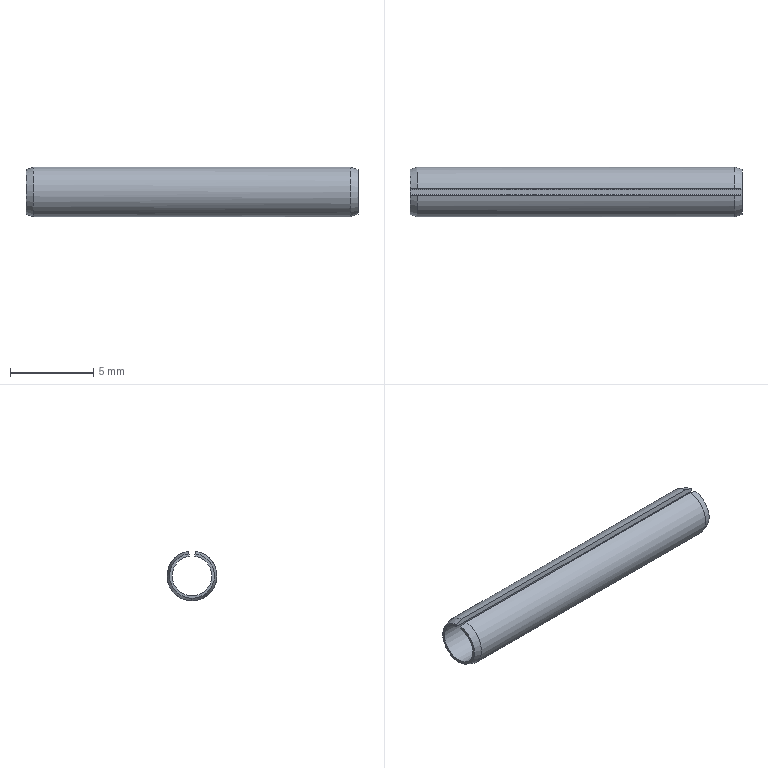Part | STEP file | spring pin slotted light duty1 gb | 1 solid | 9 faces | box 20 x 3 x 2.985 mm | volume 48.044 mm3 | plane 4 | cone 3 | cylinder 2 | commonest cylinder face diameters 2.4 x1 3 x1
STEP:
#1=CARTESIAN_POINT('',(0.,0.,0.));
#2=DIRECTION('',(0.,0.,1.));
#3=DIRECTION('',(1.,0.,0.));
#4=AXIS2_PLACEMENT_3D('',#1,#2,#3);
#5=CARTESIAN_POINT('',(0.,-0.1879,1.337));
#6=VERTEX_POINT('',#5);
#7=CARTESIAN_POINT('',(0.,0.,-1.35));
#8=VERTEX_POINT('',#7);
#9=CARTESIAN_POINT('',(0.,0.,0.));
#10=DIRECTION('',(1.,0.,0.));
#11=DIRECTION('',(0.,0.,-1.));
#12=AXIS2_PLACEMENT_3D('',#9,#10,#11);
#13=CIRCLE('',#12,1.35);
#14=CARTESIAN_POINT('',(0.,0.,0.));
#15=DIRECTION('',(1.,0.,0.));
#16=DIRECTION('',(0.,0.,-1.));
#17=AXIS2_PLACEMENT_3D('',#14,#15,#16);
#18=CONICAL_SURFACE('',#17,1.35,0.3218);
#19=CARTESIAN_POINT('',(0.,0.));
#20=DIRECTION('',(1.,0.));
#21=VECTOR('',#20,1.);
#22=LINE('',#19,#21);
#23=(GEOMETRIC_REPRESENTATION_CONTEXT(2)PARAMETRIC_REPRESENTATION_CONTEXT()REPRESENTATION_CONTEXT('',''));
#24=DEFINITIONAL_REPRESENTATION('',(#22),#23);
#25=PCURVE('',#18,#24);
#26=CARTESIAN_POINT('',(0.,0.,0.));
#27=DIRECTION('',(1.,0.,0.));
#28=DIRECTION('',(0.,0.,-1.));
#29=AXIS2_PLACEMENT_3D('',#26,#27,#28);
#30=PLANE('',#29);
#31=CARTESIAN_POINT('',(0.,0.));
#32=DIRECTION('',(1.,0.));
#33=AXIS2_PLACEMENT_2D('',#31,#32);
#34=CIRCLE('',#33,1.35);
#35=(GEOMETRIC_REPRESENTATION_CONTEXT(2)PARAMETRIC_REPRESENTATION_CONTEXT()REPRESENTATION_CONTEXT('',''));
#36=DEFINITIONAL_REPRESENTATION('',(#34),#35);
#37=PCURVE('',#30,#36);
#38=SURFACE_CURVE('',#13,(#25,#37),.PCURVE_S1.);
#39=EDGE_CURVE('',#6,#8,#38,.T.);
#40=ORIENTED_EDGE('',*,*,#39,.T.);
#41=CARTESIAN_POINT('',(0.45,0.,-1.5));
#42=VERTEX_POINT('',#41);
#43=CARTESIAN_POINT('',(0.,0.,-1.35));
#44=DIRECTION('',(0.9487,0.,-0.3162));
#45=VECTOR('',#44,1.);
#46=LINE('',#43,#45);
#47=CARTESIAN_POINT('',(6.283,0.));
#48=DIRECTION('',(0.,1.));
#49=VECTOR('',#48,1.);
#50=LINE('',#47,#49);
#51=(GEOMETRIC_REPRESENTATION_CONTEXT(2)PARAMETRIC_REPRESENTATION_CONTEXT()REPRESENTATION_CONTEXT('',''));
#52=DEFINITIONAL_REPRESENTATION('',(#50),#51);
#53=PCURVE('',#18,#52);
#54=CARTESIAN_POINT('',(0.,0.,0.));
#55=DIRECTION('',(1.,0.,0.));
#56=DIRECTION('',(0.,0.,-1.));
#57=AXIS2_PLACEMENT_3D('',#54,#55,#56);
#58=CONICAL_SURFACE('',#57,1.35,0.3218);
#59=CARTESIAN_POINT('',(0.,0.));
#60=DIRECTION('',(0.,1.));
#61=VECTOR('',#60,1.);
#62=LINE('',#59,#61);
#63=(GEOMETRIC_REPRESENTATION_CONTEXT(2)PARAMETRIC_REPRESENTATION_CONTEXT()REPRESENTATION_CONTEXT('',''));
#64=DEFINITIONAL_REPRESENTATION('',(#62),#63);
#65=PCURVE('',#58,#64);
#66=SURFACE_CURVE('',#46,(#53,#65),.PCURVE_S1.);
#67=EDGE_CURVE('',#8,#42,#66,.T.);
#68=ORIENTED_EDGE('',*,*,#67,.T.);
#69=CARTESIAN_POINT('',(0.45,-0.2088,1.485));
#70=VERTEX_POINT('',#69);
#71=CARTESIAN_POINT('',(0.45,0.,0.));
#72=DIRECTION('',(1.,0.,0.));
#73=DIRECTION('',(0.,0.,-1.));
#74=AXIS2_PLACEMENT_3D('',#71,#72,#73);
#75=CIRCLE('',#74,1.5);
#76=CARTESIAN_POINT('',(0.,0.45));
#77=DIRECTION('',(1.,0.));
#78=VECTOR('',#77,1.);
#79=LINE('',#76,#78);
#80=(GEOMETRIC_REPRESENTATION_CONTEXT(2)PARAMETRIC_REPRESENTATION_CONTEXT()REPRESENTATION_CONTEXT('',''));
#81=DEFINITIONAL_REPRESENTATION('',(#79),#80);
#82=PCURVE('',#18,#81);
#83=CARTESIAN_POINT('',(20.,0.,0.));
#84=DIRECTION('',(-1.,0.,0.));
#85=DIRECTION('',(0.,0.,1.));
#86=AXIS2_PLACEMENT_3D('',#83,#84,#85);
#87=CYLINDRICAL_SURFACE('',#86,1.5);
#88=CARTESIAN_POINT('',(9.425,19.55));
#89=DIRECTION('',(-1.,0.));
#90=VECTOR('',#89,1.);
#91=LINE('',#88,#90);
#92=(GEOMETRIC_REPRESENTATION_CONTEXT(2)PARAMETRIC_REPRESENTATION_CONTEXT()REPRESENTATION_CONTEXT('',''));
#93=DEFINITIONAL_REPRESENTATION('',(#91),#92);
#94=PCURVE('',#87,#93);
#95=SURFACE_CURVE('',#75,(#82,#94),.PCURVE_S1.);
#96=EDGE_CURVE('',#70,#42,#95,.T.);
#97=ORIENTED_EDGE('',*,*,#96,.F.);
#98=CARTESIAN_POINT('',(-4.05,0.,0.));
#99=DIRECTION('',(0.9487,-0.04401,0.3132));
#100=VECTOR('',#99,1.);
#101=LINE('',#98,#100);
#102=CARTESIAN_POINT('',(3.281,-4.05));
#103=DIRECTION('',(0.,1.));
#104=VECTOR('',#103,1.);
#105=LINE('',#102,#104);
#106=(GEOMETRIC_REPRESENTATION_CONTEXT(2)PARAMETRIC_REPRESENTATION_CONTEXT()REPRESENTATION_CONTEXT('',''));
#107=DEFINITIONAL_REPRESENTATION('',(#105),#106);
#108=PCURVE('',#18,#107);
#109=CARTESIAN_POINT('',(20.,0.,0.));
#110=DIRECTION('',(0.,0.9903,0.1392));
#111=DIRECTION('',(0.,-0.1392,0.9903));
#112=AXIS2_PLACEMENT_3D('',#109,#110,#111);
#113=PLANE('',#112);
#114=CARTESIAN_POINT('',(0.,-24.05));
#115=DIRECTION('',(0.3162,0.9487));
#116=VECTOR('',#115,1.);
#117=LINE('',#114,#116);
#118=(GEOMETRIC_REPRESENTATION_CONTEXT(2)PARAMETRIC_REPRESENTATION_CONTEXT()REPRESENTATION_CONTEXT('',''));
#119=DEFINITIONAL_REPRESENTATION('',(#117),#118);
#120=PCURVE('',#113,#119);
#121=SURFACE_CURVE('',#101,(#108,#120),.PCURVE_S1.);
#122=EDGE_CURVE('',#6,#70,#121,.T.);
#123=ORIENTED_EDGE('',*,*,#122,.F.);
#124=EDGE_LOOP('',(#40,#68,#97,#123));
#125=FACE_BOUND('',#124,.T.);
#126=ADVANCED_FACE('',(#125),#18,.T.);
#127=CARTESIAN_POINT('',(20.,-0.167,1.188));
#128=VERTEX_POINT('',#127);
#129=CARTESIAN_POINT('',(20.,0.167,1.188));
#130=VERTEX_POINT('',#129);
#131=CARTESIAN_POINT('',(20.,0.,0.));
#132=DIRECTION('',(1.,0.,0.));
#133=DIRECTION('',(0.,0.,-1.));
#134=AXIS2_PLACEMENT_3D('',#131,#132,#133);
#135=CIRCLE('',#134,1.2);
#136=CARTESIAN_POINT('',(20.,0.,0.));
#137=DIRECTION('',(1.,0.,0.));
#138=DIRECTION('',(0.,0.,-1.));
#139=AXIS2_PLACEMENT_3D('',#136,#137,#138);
#140=PLANE('',#139);
#141=CARTESIAN_POINT('',(0.,0.));
#142=DIRECTION('',(1.,0.));
#143=AXIS2_PLACEMENT_2D('',#141,#142);
#144=CIRCLE('',#143,1.2);
#145=(GEOMETRIC_REPRESENTATION_CONTEXT(2)PARAMETRIC_REPRESENTATION_CONTEXT()REPRESENTATION_CONTEXT('',''));
#146=DEFINITIONAL_REPRESENTATION('',(#144),#145);
#147=PCURVE('',#140,#146);
#148=CARTESIAN_POINT('',(23.818,0.,0.));
#149=DIRECTION('',(-1.,0.,0.));
#150=DIRECTION('',(0.,0.,1.));
#151=AXIS2_PLACEMENT_3D('',#148,#149,#150);
#152=CYLINDRICAL_SURFACE('',#151,1.2);
#153=CARTESIAN_POINT('',(9.425,3.818));
#154=DIRECTION('',(-1.,0.));
#155=VECTOR('',#154,1.);
#156=LINE('',#153,#155);
#157=(GEOMETRIC_REPRESENTATION_CONTEXT(2)PARAMETRIC_REPRESENTATION_CONTEXT()REPRESENTATION_CONTEXT('',''));
#158=DEFINITIONAL_REPRESENTATION('',(#156),#157);
#159=PCURVE('',#152,#158);
#160=SURFACE_CURVE('',#135,(#147,#159),.PCURVE_S1.);
#161=EDGE_CURVE('',#128,#130,#160,.T.);
#162=ORIENTED_EDGE('',*,*,#161,.F.);
#163=CARTESIAN_POINT('',(20.,-0.1879,1.337));
#164=VERTEX_POINT('',#163);
#165=CARTESIAN_POINT('',(20.,0.,0.));
#166=DIRECTION('',(0.,0.1392,-0.9903));
#167=VECTOR('',#166,1.);
#168=LINE('',#165,#167);
#169=CARTESIAN_POINT('',(0.,0.));
#170=DIRECTION('',(0.9903,0.1392));
#171=VECTOR('',#170,1.);
#172=LINE('',#169,#171);
#173=(GEOMETRIC_REPRESENTATION_CONTEXT(2)PARAMETRIC_REPRESENTATION_CONTEXT()REPRESENTATION_CONTEXT('',''));
#174=DEFINITIONAL_REPRESENTATION('',(#172),#173);
#175=PCURVE('',#140,#174);
#176=CARTESIAN_POINT('',(0.,0.));
#177=DIRECTION('',(-1.,0.));
#178=VECTOR('',#177,1.);
#179=LINE('',#176,#178);
#180=(GEOMETRIC_REPRESENTATION_CONTEXT(2)PARAMETRIC_REPRESENTATION_CONTEXT()REPRESENTATION_CONTEXT('',''));
#181=DEFINITIONAL_REPRESENTATION('',(#179),#180);
#182=PCURVE('',#113,#181);
#183=SURFACE_CURVE('',#168,(#175,#182),.PCURVE_S1.);
#184=EDGE_CURVE('',#164,#128,#183,.T.);
#185=ORIENTED_EDGE('',*,*,#184,.F.);
#186=CARTESIAN_POINT('',(20.,0.1879,1.337));
#187=VERTEX_POINT('',#186);
#188=CARTESIAN_POINT('',(20.,0.,0.));
#189=DIRECTION('',(1.,0.,0.));
#190=DIRECTION('',(0.,0.,-1.));
#191=AXIS2_PLACEMENT_3D('',#188,#189,#190);
#192=CIRCLE('',#191,1.35);
#193=CARTESIAN_POINT('',(0.,0.));
#194=DIRECTION('',(1.,0.));
#195=AXIS2_PLACEMENT_2D('',#193,#194);
#196=CIRCLE('',#195,1.35);
#197=(GEOMETRIC_REPRESENTATION_CONTEXT(2)PARAMETRIC_REPRESENTATION_CONTEXT()REPRESENTATION_CONTEXT('',''));
#198=DEFINITIONAL_REPRESENTATION('',(#196),#197);
#199=PCURVE('',#140,#198);
#200=CARTESIAN_POINT('',(19.55,0.,0.));
#201=DIRECTION('',(-1.,0.,0.));
#202=DIRECTION('',(0.,0.,1.));
#203=AXIS2_PLACEMENT_3D('',#200,#201,#202);
#204=CONICAL_SURFACE('',#203,1.5,0.3218);
#205=CARTESIAN_POINT('',(9.425,-0.45));
#206=DIRECTION('',(-1.,0.));
#207=VECTOR('',#206,1.);
#208=LINE('',#205,#207);
#209=(GEOMETRIC_REPRESENTATION_CONTEXT(2)PARAMETRIC_REPRESENTATION_CONTEXT()REPRESENTATION_CONTEXT('',''));
#210=DEFINITIONAL_REPRESENTATION('',(#208),#209);
#211=PCURVE('',#204,#210);
#212=SURFACE_CURVE('',#192,(#199,#211),.PCURVE_S1.);
#213=EDGE_CURVE('',#164,#187,#212,.T.);
#214=ORIENTED_EDGE('',*,*,#213,.T.);
#215=CARTESIAN_POINT('',(20.,0.,0.));
#216=DIRECTION('',(0.,0.1392,0.9903));
#217=VECTOR('',#216,1.);
#218=LINE('',#215,#217);
#219=CARTESIAN_POINT('',(0.,0.));
#220=DIRECTION('',(-0.9903,0.1392));
#221=VECTOR('',#220,1.);
#222=LINE('',#219,#221);
#223=(GEOMETRIC_REPRESENTATION_CONTEXT(2)PARAMETRIC_REPRESENTATION_CONTEXT()REPRESENTATION_CONTEXT('',''));
#224=DEFINITIONAL_REPRESENTATION('',(#222),#223);
#225=PCURVE('',#140,#224);
#226=CARTESIAN_POINT('',(20.,0.,0.));
#227=DIRECTION('',(0.,-0.9903,0.1392));
#228=DIRECTION('',(0.,-0.1392,-0.9903));
#229=AXIS2_PLACEMENT_3D('',#226,#227,#228);
#230=PLANE('',#229);
#231=CARTESIAN_POINT('',(0.,0.));
#232=DIRECTION('',(-1.,0.));
#233=VECTOR('',#232,1.);
#234=LINE('',#231,#233);
#235=(GEOMETRIC_REPRESENTATION_CONTEXT(2)PARAMETRIC_REPRESENTATION_CONTEXT()REPRESENTATION_CONTEXT('',''));
#236=DEFINITIONAL_REPRESENTATION('',(#234),#235);
#237=PCURVE('',#230,#236);
#238=SURFACE_CURVE('',#218,(#225,#237),.PCURVE_S1.);
#239=EDGE_CURVE('',#130,#187,#238,.T.);
#240=ORIENTED_EDGE('',*,*,#239,.F.);
#241=EDGE_LOOP('',(#162,#185,#214,#240));
#242=FACE_BOUND('',#241,.T.);
#243=ADVANCED_FACE('',(#242),#140,.T.);
#244=CARTESIAN_POINT('',(0.,-0.167,1.188));
#245=VERTEX_POINT('',#244);
#246=CARTESIAN_POINT('',(0.,0.,0.));
#247=DIRECTION('',(0.,0.1392,-0.9903));
#248=VECTOR('',#247,1.);
#249=LINE('',#246,#248);
#250=CARTESIAN_POINT('',(0.,0.));
#251=DIRECTION('',(0.9903,0.1392));
#252=VECTOR('',#251,1.);
#253=LINE('',#250,#252);
#254=(GEOMETRIC_REPRESENTATION_CONTEXT(2)PARAMETRIC_REPRESENTATION_CONTEXT()REPRESENTATION_CONTEXT('',''));
#255=DEFINITIONAL_REPRESENTATION('',(#253),#254);
#256=PCURVE('',#30,#255);
#257=CARTESIAN_POINT('',(0.,-20.));
#258=DIRECTION('',(-1.,0.));
#259=VECTOR('',#258,1.);
#260=LINE('',#257,#259);
#261=(GEOMETRIC_REPRESENTATION_CONTEXT(2)PARAMETRIC_REPRESENTATION_CONTEXT()REPRESENTATION_CONTEXT('',''));
#262=DEFINITIONAL_REPRESENTATION('',(#260),#261);
#263=PCURVE('',#113,#262);
#264=SURFACE_CURVE('',#249,(#256,#263),.PCURVE_S1.);
#265=EDGE_CURVE('',#6,#245,#264,.T.);
#266=ORIENTED_EDGE('',*,*,#265,.T.);
#267=CARTESIAN_POINT('',(0.,0.167,1.188));
#268=VERTEX_POINT('',#267);
#269=CARTESIAN_POINT('',(0.,0.,0.));
#270=DIRECTION('',(1.,0.,0.));
#271=DIRECTION('',(0.,0.,-1.));
#272=AXIS2_PLACEMENT_3D('',#269,#270,#271);
#273=CIRCLE('',#272,1.2);
#274=CARTESIAN_POINT('',(0.,0.));
#275=DIRECTION('',(1.,0.));
#276=AXIS2_PLACEMENT_2D('',#274,#275);
#277=CIRCLE('',#276,1.2);
#278=(GEOMETRIC_REPRESENTATION_CONTEXT(2)PARAMETRIC_REPRESENTATION_CONTEXT()REPRESENTATION_CONTEXT('',''));
#279=DEFINITIONAL_REPRESENTATION('',(#277),#278);
#280=PCURVE('',#30,#279);
#281=CARTESIAN_POINT('',(9.425,23.818));
#282=DIRECTION('',(-1.,0.));
#283=VECTOR('',#282,1.);
#284=LINE('',#281,#283);
#285=(GEOMETRIC_REPRESENTATION_CONTEXT(2)PARAMETRIC_REPRESENTATION_CONTEXT()REPRESENTATION_CONTEXT('',''));
#286=DEFINITIONAL_REPRESENTATION('',(#284),#285);
#287=PCURVE('',#152,#286);
#288=SURFACE_CURVE('',#273,(#280,#287),.PCURVE_S1.);
#289=EDGE_CURVE('',#245,#268,#288,.T.);
#290=ORIENTED_EDGE('',*,*,#289,.T.);
#291=CARTESIAN_POINT('',(0.,0.1879,1.337));
#292=VERTEX_POINT('',#291);
#293=CARTESIAN_POINT('',(0.,0.,0.));
#294=DIRECTION('',(0.,0.1392,0.9903));
#295=VECTOR('',#294,1.);
#296=LINE('',#293,#295);
#297=CARTESIAN_POINT('',(0.,0.));
#298=DIRECTION('',(-0.9903,0.1392));
#299=VECTOR('',#298,1.);
#300=LINE('',#297,#299);
#301=(GEOMETRIC_REPRESENTATION_CONTEXT(2)PARAMETRIC_REPRESENTATION_CONTEXT()REPRESENTATION_CONTEXT('',''));
#302=DEFINITIONAL_REPRESENTATION('',(#300),#301);
#303=PCURVE('',#30,#302);
#304=CARTESIAN_POINT('',(0.,-20.));
#305=DIRECTION('',(-1.,0.));
#306=VECTOR('',#305,1.);
#307=LINE('',#304,#306);
#308=(GEOMETRIC_REPRESENTATION_CONTEXT(2)PARAMETRIC_REPRESENTATION_CONTEXT()REPRESENTATION_CONTEXT('',''));
#309=DEFINITIONAL_REPRESENTATION('',(#307),#308);
#310=PCURVE('',#230,#309);
#311=SURFACE_CURVE('',#296,(#303,#310),.PCURVE_S1.);
#312=EDGE_CURVE('',#268,#292,#311,.T.);
#313=ORIENTED_EDGE('',*,*,#312,.T.);
#314=CARTESIAN_POINT('',(0.,0.,0.));
#315=DIRECTION('',(1.,0.,0.));
#316=DIRECTION('',(0.,0.,-1.));
#317=AXIS2_PLACEMENT_3D('',#314,#315,#316);
#318=CIRCLE('',#317,1.35);
#319=CARTESIAN_POINT('',(0.,0.));
#320=DIRECTION('',(1.,0.));
#321=AXIS2_PLACEMENT_2D('',#319,#320);
#322=CIRCLE('',#321,1.35);
#323=(GEOMETRIC_REPRESENTATION_CONTEXT(2)PARAMETRIC_REPRESENTATION_CONTEXT()REPRESENTATION_CONTEXT('',''));
#324=DEFINITIONAL_REPRESENTATION('',(#322),#323);
#325=PCURVE('',#30,#324);
#326=CARTESIAN_POINT('',(0.,0.));
#327=DIRECTION('',(1.,0.));
#328=VECTOR('',#327,1.);
#329=LINE('',#326,#328);
#330=(GEOMETRIC_REPRESENTATION_CONTEXT(2)PARAMETRIC_REPRESENTATION_CONTEXT()REPRESENTATION_CONTEXT('',''));
#331=DEFINITIONAL_REPRESENTATION('',(#329),#330);
#332=PCURVE('',#58,#331);
#333=SURFACE_CURVE('',#318,(#325,#332),.PCURVE_S1.);
#334=EDGE_CURVE('',#8,#292,#333,.T.);
#335=ORIENTED_EDGE('',*,*,#334,.F.);
#336=ORIENTED_EDGE('',*,*,#39,.F.);
#337=EDGE_LOOP('',(#266,#290,#313,#335,#336));
#338=FACE_BOUND('',#337,.T.);
#339=ADVANCED_FACE('',(#338),#30,.F.);
#340=CARTESIAN_POINT('',(19.55,-0.2088,1.485));
#341=VERTEX_POINT('',#340);
#342=CARTESIAN_POINT('',(20.,-0.2088,1.485));
#343=DIRECTION('',(1.,0.,0.));
#344=VECTOR('',#343,1.);
#345=LINE('',#342,#344);
#346=CARTESIAN_POINT('',(6.144,0.));
#347=DIRECTION('',(0.,-1.));
#348=VECTOR('',#347,1.);
#349=LINE('',#346,#348);
#350=(GEOMETRIC_REPRESENTATION_CONTEXT(2)PARAMETRIC_REPRESENTATION_CONTEXT()REPRESENTATION_CONTEXT('',''));
#351=DEFINITIONAL_REPRESENTATION('',(#349),#350);
#352=PCURVE('',#87,#351);
#353=CARTESIAN_POINT('',(1.5,0.));
#354=DIRECTION('',(0.,1.));
#355=VECTOR('',#354,1.);
#356=LINE('',#353,#355);
#357=(GEOMETRIC_REPRESENTATION_CONTEXT(2)PARAMETRIC_REPRESENTATION_CONTEXT()REPRESENTATION_CONTEXT('',''));
#358=DEFINITIONAL_REPRESENTATION('',(#356),#357);
#359=PCURVE('',#113,#358);
#360=SURFACE_CURVE('',#345,(#352,#359),.PCURVE_S1.);
#361=EDGE_CURVE('',#70,#341,#360,.T.);
#362=ORIENTED_EDGE('',*,*,#361,.F.);
#363=ORIENTED_EDGE('',*,*,#96,.T.);
#364=CARTESIAN_POINT('',(0.45,0.2088,1.485));
#365=VERTEX_POINT('',#364);
#366=CARTESIAN_POINT('',(0.45,0.,0.));
#367=DIRECTION('',(1.,0.,0.));
#368=DIRECTION('',(0.,0.,-1.));
#369=AXIS2_PLACEMENT_3D('',#366,#367,#368);
#370=CIRCLE('',#369,1.5);
#371=CARTESIAN_POINT('',(3.142,19.55));
#372=DIRECTION('',(-1.,0.));
#373=VECTOR('',#372,1.);
#374=LINE('',#371,#373);
#375=(GEOMETRIC_REPRESENTATION_CONTEXT(2)PARAMETRIC_REPRESENTATION_CONTEXT()REPRESENTATION_CONTEXT('',''));
#376=DEFINITIONAL_REPRESENTATION('',(#374),#375);
#377=PCURVE('',#87,#376);
#378=CARTESIAN_POINT('',(0.,0.45));
#379=DIRECTION('',(1.,0.));
#380=VECTOR('',#379,1.);
#381=LINE('',#378,#380);
#382=(GEOMETRIC_REPRESENTATION_CONTEXT(2)PARAMETRIC_REPRESENTATION_CONTEXT()REPRESENTATION_CONTEXT('',''));
#383=DEFINITIONAL_REPRESENTATION('',(#381),#382);
#384=PCURVE('',#58,#383);
#385=SURFACE_CURVE('',#370,(#377,#384),.PCURVE_S1.);
#386=EDGE_CURVE('',#42,#365,#385,.T.);
#387=ORIENTED_EDGE('',*,*,#386,.T.);
#388=CARTESIAN_POINT('',(19.55,0.2088,1.485));
#389=VERTEX_POINT('',#388);
#390=CARTESIAN_POINT('',(20.,0.2088,1.485));
#391=DIRECTION('',(-1.,0.,0.));
#392=VECTOR('',#391,1.);
#393=LINE('',#390,#392);
#394=CARTESIAN_POINT('',(0.1396,0.));
#395=DIRECTION('',(0.,1.));
#396=VECTOR('',#395,1.);
#397=LINE('',#394,#396);
#398=(GEOMETRIC_REPRESENTATION_CONTEXT(2)PARAMETRIC_REPRESENTATION_CONTEXT()REPRESENTATION_CONTEXT('',''));
#399=DEFINITIONAL_REPRESENTATION('',(#397),#398);
#400=PCURVE('',#87,#399);
#401=CARTESIAN_POINT('',(-1.5,0.));
#402=DIRECTION('',(0.,-1.));
#403=VECTOR('',#402,1.);
#404=LINE('',#401,#403);
#405=(GEOMETRIC_REPRESENTATION_CONTEXT(2)PARAMETRIC_REPRESENTATION_CONTEXT()REPRESENTATION_CONTEXT('',''));
#406=DEFINITIONAL_REPRESENTATION('',(#404),#405);
#407=PCURVE('',#230,#406);
#408=SURFACE_CURVE('',#393,(#400,#407),.PCURVE_S1.);
#409=EDGE_CURVE('',#389,#365,#408,.T.);
#410=ORIENTED_EDGE('',*,*,#409,.F.);
#411=CARTESIAN_POINT('',(19.55,0.,0.));
#412=DIRECTION('',(1.,0.,0.));
#413=DIRECTION('',(0.,0.,-1.));
#414=AXIS2_PLACEMENT_3D('',#411,#412,#413);
#415=CIRCLE('',#414,1.5);
#416=CARTESIAN_POINT('',(9.425,0.45));
#417=DIRECTION('',(-1.,0.));
#418=VECTOR('',#417,1.);
#419=LINE('',#416,#418);
#420=(GEOMETRIC_REPRESENTATION_CONTEXT(2)PARAMETRIC_REPRESENTATION_CONTEXT()REPRESENTATION_CONTEXT('',''));
#421=DEFINITIONAL_REPRESENTATION('',(#419),#420);
#422=PCURVE('',#87,#421);
#423=CARTESIAN_POINT('',(9.425,0.));
#424=DIRECTION('',(-1.,0.));
#425=VECTOR('',#424,1.);
#426=LINE('',#423,#425);
#427=(GEOMETRIC_REPRESENTATION_CONTEXT(2)PARAMETRIC_REPRESENTATION_CONTEXT()REPRESENTATION_CONTEXT('',''));
#428=DEFINITIONAL_REPRESENTATION('',(#426),#427);
#429=PCURVE('',#204,#428);
#430=SURFACE_CURVE('',#415,(#422,#429),.PCURVE_S1.);
#431=EDGE_CURVE('',#341,#389,#430,.T.);
#432=ORIENTED_EDGE('',*,*,#431,.F.);
#433=EDGE_LOOP('',(#362,#363,#387,#410,#432));
#434=FACE_BOUND('',#433,.T.);
#435=ADVANCED_FACE('',(#434),#87,.T.);
#436=CARTESIAN_POINT('',(23.818,0.167,1.188));
#437=DIRECTION('',(-1.,0.,0.));
#438=VECTOR('',#437,1.);
#439=LINE('',#436,#438);
#440=CARTESIAN_POINT('',(0.1396,0.));
#441=DIRECTION('',(0.,1.));
#442=VECTOR('',#441,1.);
#443=LINE('',#440,#442);
#444=(GEOMETRIC_REPRESENTATION_CONTEXT(2)PARAMETRIC_REPRESENTATION_CONTEXT()REPRESENTATION_CONTEXT('',''));
#445=DEFINITIONAL_REPRESENTATION('',(#443),#444);
#446=PCURVE('',#152,#445);
#447=CARTESIAN_POINT('',(-1.2,3.818));
#448=DIRECTION('',(0.,-1.));
#449=VECTOR('',#448,1.);
#450=LINE('',#447,#449);
#451=(GEOMETRIC_REPRESENTATION_CONTEXT(2)PARAMETRIC_REPRESENTATION_CONTEXT()REPRESENTATION_CONTEXT('',''));
#452=DEFINITIONAL_REPRESENTATION('',(#450),#451);
#453=PCURVE('',#230,#452);
#454=SURFACE_CURVE('',#439,(#446,#453),.PCURVE_S1.);
#455=EDGE_CURVE('',#130,#268,#454,.T.);
#456=ORIENTED_EDGE('',*,*,#455,.F.);
#457=ORIENTED_EDGE('',*,*,#161,.F.);
#458=CARTESIAN_POINT('',(23.818,-0.167,1.188));
#459=DIRECTION('',(1.,0.,0.));
#460=VECTOR('',#459,1.);
#461=LINE('',#458,#460);
#462=CARTESIAN_POINT('',(6.144,0.));
#463=DIRECTION('',(0.,-1.));
#464=VECTOR('',#463,1.);
#465=LINE('',#462,#464);
#466=(GEOMETRIC_REPRESENTATION_CONTEXT(2)PARAMETRIC_REPRESENTATION_CONTEXT()REPRESENTATION_CONTEXT('',''));
#467=DEFINITIONAL_REPRESENTATION('',(#465),#466);
#468=PCURVE('',#152,#467);
#469=CARTESIAN_POINT('',(1.2,3.818));
#470=DIRECTION('',(0.,1.));
#471=VECTOR('',#470,1.);
#472=LINE('',#469,#471);
#473=(GEOMETRIC_REPRESENTATION_CONTEXT(2)PARAMETRIC_REPRESENTATION_CONTEXT()REPRESENTATION_CONTEXT('',''));
#474=DEFINITIONAL_REPRESENTATION('',(#472),#473);
#475=PCURVE('',#113,#474);
#476=SURFACE_CURVE('',#461,(#468,#475),.PCURVE_S1.);
#477=EDGE_CURVE('',#245,#128,#476,.T.);
#478=ORIENTED_EDGE('',*,*,#477,.F.);
#479=ORIENTED_EDGE('',*,*,#289,.T.);
#480=EDGE_LOOP('',(#456,#457,#478,#479));
#481=FACE_BOUND('',#480,.F.);
#482=ADVANCED_FACE('',(#481),#152,.F.);
#483=CARTESIAN_POINT('',(24.05,0.,0.));
#484=DIRECTION('',(0.9487,0.04401,-0.3132));
#485=VECTOR('',#484,1.);
#486=LINE('',#483,#485);
#487=CARTESIAN_POINT('',(6.144,-4.5));
#488=DIRECTION('',(0.,-1.));
#489=VECTOR('',#488,1.);
#490=LINE('',#487,#489);
#491=(GEOMETRIC_REPRESENTATION_CONTEXT(2)PARAMETRIC_REPRESENTATION_CONTEXT()REPRESENTATION_CONTEXT('',''));
#492=DEFINITIONAL_REPRESENTATION('',(#490),#491);
#493=PCURVE('',#204,#492);
#494=CARTESIAN_POINT('',(0.,4.05));
#495=DIRECTION('',(-0.3162,0.9487));
#496=VECTOR('',#495,1.);
#497=LINE('',#494,#496);
#498=(GEOMETRIC_REPRESENTATION_CONTEXT(2)PARAMETRIC_REPRESENTATION_CONTEXT()REPRESENTATION_CONTEXT('',''));
#499=DEFINITIONAL_REPRESENTATION('',(#497),#498);
#500=PCURVE('',#113,#499);
#501=SURFACE_CURVE('',#486,(#493,#500),.PCURVE_S1.);
#502=EDGE_CURVE('',#341,#164,#501,.T.);
#503=ORIENTED_EDGE('',*,*,#502,.F.);
#504=ORIENTED_EDGE('',*,*,#431,.T.);
#505=CARTESIAN_POINT('',(24.05,0.,0.));
#506=DIRECTION('',(-0.9487,0.04401,0.3132));
#507=VECTOR('',#506,1.);
#508=LINE('',#505,#507);
#509=CARTESIAN_POINT('',(0.1396,-4.5));
#510=DIRECTION('',(0.,1.));
#511=VECTOR('',#510,1.);
#512=LINE('',#509,#511);
#513=(GEOMETRIC_REPRESENTATION_CONTEXT(2)PARAMETRIC_REPRESENTATION_CONTEXT()REPRESENTATION_CONTEXT('',''));
#514=DEFINITIONAL_REPRESENTATION('',(#512),#513);
#515=PCURVE('',#204,#514);
#516=CARTESIAN_POINT('',(0.,4.05));
#517=DIRECTION('',(-0.3162,-0.9487));
#518=VECTOR('',#517,1.);
#519=LINE('',#516,#518);
#520=(GEOMETRIC_REPRESENTATION_CONTEXT(2)PARAMETRIC_REPRESENTATION_CONTEXT()REPRESENTATION_CONTEXT('',''));
#521=DEFINITIONAL_REPRESENTATION('',(#519),#520);
#522=PCURVE('',#230,#521);
#523=SURFACE_CURVE('',#508,(#515,#522),.PCURVE_S1.);
#524=EDGE_CURVE('',#187,#389,#523,.T.);
#525=ORIENTED_EDGE('',*,*,#524,.F.);
#526=ORIENTED_EDGE('',*,*,#213,.F.);
#527=EDGE_LOOP('',(#503,#504,#525,#526));
#528=FACE_BOUND('',#527,.T.);
#529=ADVANCED_FACE('',(#528),#204,.T.);
#530=ORIENTED_EDGE('',*,*,#67,.F.);
#531=ORIENTED_EDGE('',*,*,#334,.T.);
#532=CARTESIAN_POINT('',(-4.05,0.,0.));
#533=DIRECTION('',(-0.9487,-0.04401,-0.3132));
#534=VECTOR('',#533,1.);
#535=LINE('',#532,#534);
#536=CARTESIAN_POINT('',(3.002,-4.05));
#537=DIRECTION('',(0.,-1.));
#538=VECTOR('',#537,1.);
#539=LINE('',#536,#538);
#540=(GEOMETRIC_REPRESENTATION_CONTEXT(2)PARAMETRIC_REPRESENTATION_CONTEXT()REPRESENTATION_CONTEXT('',''));
#541=DEFINITIONAL_REPRESENTATION('',(#539),#540);
#542=PCURVE('',#58,#541);
#543=CARTESIAN_POINT('',(0.,-24.05));
#544=DIRECTION('',(0.3162,-0.9487));
#545=VECTOR('',#544,1.);
#546=LINE('',#543,#545);
#547=(GEOMETRIC_REPRESENTATION_CONTEXT(2)PARAMETRIC_REPRESENTATION_CONTEXT()REPRESENTATION_CONTEXT('',''));
#548=DEFINITIONAL_REPRESENTATION('',(#546),#547);
#549=PCURVE('',#230,#548);
#550=SURFACE_CURVE('',#535,(#542,#549),.PCURVE_S1.);
#551=EDGE_CURVE('',#365,#292,#550,.T.);
#552=ORIENTED_EDGE('',*,*,#551,.F.);
#553=ORIENTED_EDGE('',*,*,#386,.F.);
#554=EDGE_LOOP('',(#530,#531,#552,#553));
#555=FACE_BOUND('',#554,.T.);
#556=ADVANCED_FACE('',(#555),#58,.T.);
#557=ORIENTED_EDGE('',*,*,#239,.T.);
#558=ORIENTED_EDGE('',*,*,#524,.T.);
#559=ORIENTED_EDGE('',*,*,#409,.T.);
#560=ORIENTED_EDGE('',*,*,#551,.T.);
#561=ORIENTED_EDGE('',*,*,#312,.F.);
#562=ORIENTED_EDGE('',*,*,#455,.F.);
#563=EDGE_LOOP('',(#557,#558,#559,#560,#561,#562));
#564=FACE_BOUND('',#563,.T.);
#565=ADVANCED_FACE('',(#564),#230,.T.);
#566=ORIENTED_EDGE('',*,*,#265,.F.);
#567=ORIENTED_EDGE('',*,*,#122,.T.);
#568=ORIENTED_EDGE('',*,*,#361,.T.);
#569=ORIENTED_EDGE('',*,*,#502,.T.);
#570=ORIENTED_EDGE('',*,*,#184,.T.);
#571=ORIENTED_EDGE('',*,*,#477,.F.);
#572=EDGE_LOOP('',(#566,#567,#568,#569,#570,#571));
#573=FACE_BOUND('',#572,.T.);
#574=ADVANCED_FACE('',(#573),#113,.T.);
#575=CLOSED_SHELL('',(#126,#243,#339,#435,#482,#529,#556,#565,#574));
#576=MANIFOLD_SOLID_BREP('',#575);
#577=(LENGTH_UNIT()NAMED_UNIT(*)SI_UNIT(.MILLI.,.METRE.));
#578=UNCERTAINTY_MEASURE_WITH_UNIT(LENGTH_MEASURE(0.0000001),#577,'','');
#579=(NAMED_UNIT(*)PLANE_ANGLE_UNIT()SI_UNIT($,.RADIAN.));
#580=(NAMED_UNIT(*)SI_UNIT($,.STERADIAN.)SOLID_ANGLE_UNIT());
#581=(GEOMETRIC_REPRESENTATION_CONTEXT(3)GLOBAL_UNCERTAINTY_ASSIGNED_CONTEXT((#578))GLOBAL_UNIT_ASSIGNED_CONTEXT((#577,#579,#580))REPRESENTATION_CONTEXT('',''));
#582=ADVANCED_BREP_SHAPE_REPRESENTATION('',(#4,#576),#581);